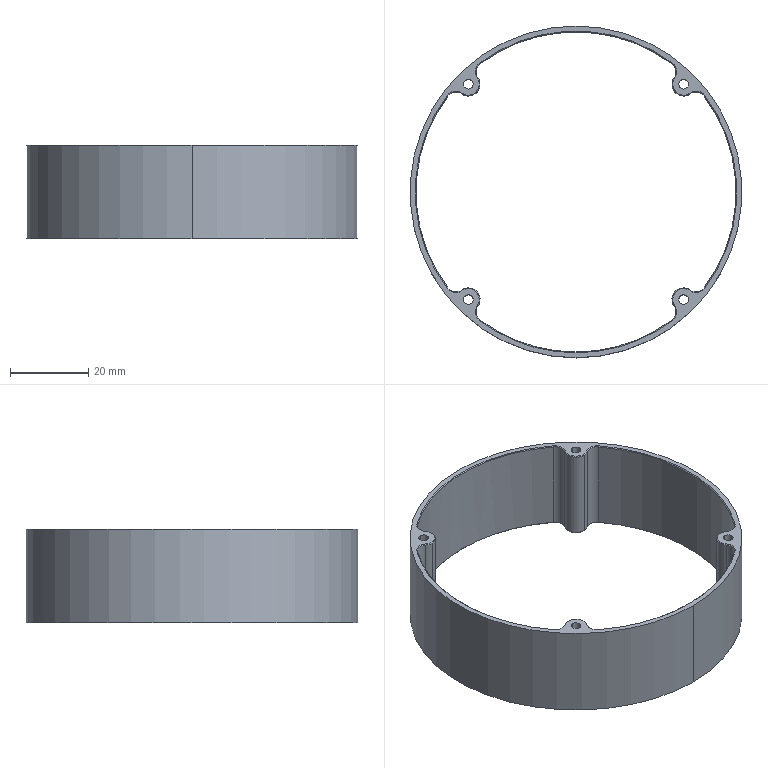NC program | NX | posted with a generic post | part box 85 x 85 x 24 mm
Whole program:
N10 G17 G21 G94 G90
(FLOOR_WALL , TOOL : D80)
N12 T19 M6
N14 G54
N16 G17 G0 G90 X-90.5 Y47.497 S6500 M3
N18 G43 Z30. H19
N20 Z3.
N22 G94 G1 Z0. F1500.
N24 X-87.5
N26 X87.5
N28 Y-15.5
N30 X-87.5
N32 X-90.5
N34 Z3.
N36 G0 Z30.
N38 M5
(ADAPTIVE_MILLING , TOOL : D10)
N40 T15 M6
N42 G54
N44 G17 G0 G90 X-55.209 Y0.813 S9500 M3
N46 G43 Z30. H15
N48 Z-21.
N50 G94 G1 Z-24. F1000.
N52 X-54.429 Y0.533 F3000.
N54 X-53.64 Y0.277
N56 G3 X-52.562 Y0.813 R1.017
N58 X-51.801 Y3.876 R8.28
N60 X-51.519 Y13.744 R111.643
N62 G1 X-51.514 Y15.994
N64 X-51.511 Y19.869
N66 X-51.51 Y33.494
N68 Y44.369
N70 X-51.509 Y44.494
N72 X-51.508 Y44.618
N74 G2 X-49.014 Y48.899 R5.714
N76 X-43.574 Y50.965 R12.318
N78 X-35.346 Y51.454 R58.245
N80 G1 X-34.346 Y51.464
N82 X-33.096 Y51.472
N84 X-31.347 Y51.48
N86 X-29.097 Y51.485
N88 X-25.222 Y51.487
N90 X-10.472 Y51.488
N92 X34.403
N94 X35.153 Y51.492
N96 X36.278 Y51.494
N98 X37.153
N100 X37.903 Y51.496
N102 X39.028
N104 G2 X45.027 Y51.463 R213.622
N106 X49.208 Y48.563 R6.076
N108 X51.082 Y42.786 R13.838
N110 X51.47 Y33.674 R81.696
N112 G1 X51.477 Y32.174
N114 X51.483 Y30.174
N116 X51.486 Y27.174
N118 X51.488 Y20.424
N120 Y-44.576
N122 X51.484 Y-44.701
N124 G2 X48.93 Y-48.952 R5.793
N126 X43.474 Y-50.979 R12.522
N128 X35.245 Y-51.455 R59.636
N130 G1 X34.12 Y-51.466
N132 X32.995 Y-51.473
N134 X31.495 Y-51.479
N136 X29.245 Y-51.484
N138 X25.495 Y-51.487
N140 X12.745 Y-51.488
N142 X-44.505
N144 X-44.63 Y-51.486
N146 X-44.755 Y-51.48
N148 X-44.879 Y-51.471
N150 G2 X-49.054 Y-48.781 R5.933
N152 X-51.022 Y-43.17 R12.937
N154 X-51.464 Y-34.313 R70.547
N156 G1 X-51.473 Y-33.063
N158 X-51.479 Y-31.438
N160 X-51.484 Y-29.063
N162 X-51.487 Y-25.188
N164 X-51.488 Y-11.938
N166 Y-2.938
N168 G2 X-50.952 Y2.659 R65.706
N170 G3 X-50.542 Y13.772 R121.144
N172 G1 X-50.534 Y15.397
N174 X-50.528 Y17.522
N176 X-50.523 Y20.647
N178 X-50.521 Y26.647
N180 Y41.397
N182 X-50.519 Y41.522
N184 G2 X-46.822 Y47.831 R7.658
N186 X-40.599 Y49.949 R15.406
N188 X-31.994 Y50.437 R67.483
N190 G1 X-30.869 Y50.449
N192 X-29.619 Y50.458
N194 X-27.994 Y50.466
N196 X-25.869 Y50.472
N198 X-22.619 Y50.476
N200 X-15.619 Y50.478
N202 X31.381
N204 X32.256 Y50.482
N206 X33.381 Y50.485
N208 X34.256
N210 X35.006 Y50.489
N212 X36.131 Y50.491
N214 G2 X42.254 Y50.449 R121.112
N216 X47.892 Y46.712 R7.759
N218 X49.996 Y40.224 R15.82
N220 X50.448 Y30.991 R77.748
N222 G1 X50.458 Y29.741
N224 X50.466 Y28.116
N226 X50.472 Y25.991
N228 X50.475 Y22.866
N230 X50.477 Y16.366
N232 X50.478 Y-41.384
N234 G2 X46.906 Y-47.756 R7.572
N236 X40.829 Y-49.911 R14.905
N238 X32.226 Y-50.433 R63.965
N240 G1 X31.226 Y-50.445
N242 X29.976 Y-50.455
N244 X28.476 Y-50.464
N246 X26.851 Y-50.469
N248 X24.227 Y-50.474
N250 X19.602 Y-50.477
N252 X-5.523 Y-50.478
N254 X-41.398
N256 X-41.523 Y-50.477
N258 X-41.648 Y-50.474
N260 X-41.773 Y-50.469
N262 X-41.898 Y-50.463
N264 G2 X-47.966 Y-46.571 R7.736
N266 X-49.986 Y-40.312 R16.029
N268 X-50.447 Y-30.954 R79.258
N270 G1 X-50.456 Y-29.829
N272 X-50.464 Y-28.454
N274 X-50.47 Y-26.454
N276 X-50.474 Y-23.704
N278 X-50.477 Y-18.704
N280 X-50.478 Y-5.329
N282 G2 X-49.974 Y2.402 R101.984
N284 G3 X-49.542 Y18.267 R208.612
N286 G1 X-49.536 Y21.017
N288 X-49.533 Y25.267
N290 X-49.532 Y36.142
N292 Y38.392
N294 X-49.53 Y38.767
N296 X-49.528 Y38.892
N298 G2 X-44.723 Y46.953 R8.987
N300 X-37.94 Y48.979 R18.304
N302 X-27.206 Y49.443 R96.865
N304 G1 X-25.706 Y49.451
N306 X-23.706 Y49.458
N308 X-20.956 Y49.463
N310 X-16.456 Y49.466
N312 X1.169 Y49.467
N314 X28.419
N316 G2 X39.793 Y49.452 R397.8
N318 X46.908 Y44.779 R8.926
N320 X48.996 Y37.758 R18.255
N322 X49.439 Y27.648 R96.534
N324 G1 X49.448 Y26.398
N326 X49.455 Y24.773
N328 X49.461 Y22.523
N330 X49.465 Y19.148
N332 X49.467 Y12.148
N334 Y-38.727
N336 G2 X44.822 Y-46.874 R8.92
N338 X37.934 Y-48.972 R17.859
N340 X27.451 Y-49.44 R95.726
N342 G1 X26.076 Y-49.449
N344 X24.326 Y-49.456
N346 X21.951 Y-49.462
N348 X18.201 Y-49.465
N350 X9.451 Y-49.467
N352 X-38.799
N354 G2 X-46.91 Y-44.755 R8.939
N356 X-48.964 Y-37.982 R17.998
N358 X-49.437 Y-27.749 R91.373
N360 G1 X-49.446 Y-26.624
N362 X-49.454 Y-24.999
N364 X-49.46 Y-22.874
N366 X-49.464 Y-19.874
N368 X-49.466 Y-14.124
N370 X-49.467 Y-7.124
N372 G2 X-49.015 Y1.737 R130.332
N374 G3 X-48.553 Y20.103 R271.383
N376 G1 X-48.547 Y23.103
N378 X-48.544 Y27.853
N380 X-48.542 Y35.353
N382 X-48.538 Y36.103
N384 X-48.531 Y36.728
N386 X-48.525 Y36.978
N388 G2 X-42.997 Y45.963 R9.907
N390 X-35.568 Y48.004 R20.654
N392 X-24.706 Y48.431 R112.646
N394 G1 X-23.081 Y48.44
N396 X-21.081 Y48.447
N398 X-18.331 Y48.452
N400 X-13.956 Y48.455
N402 X-0.706 Y48.456
N404 X25.419
N406 G2 X37.793 Y48.44 R387.041
N408 X45.938 Y43.012 R9.811
N410 X47.951 Y35.961 R20.187
N412 X48.43 Y24.727 R104.006
N414 G1 X48.44 Y23.102
N416 X48.446 Y21.477
N418 X48.451 Y19.102
N420 X48.455 Y15.102
N422 X48.456 Y5.227
N424 Y-36.398
N426 G2 X46.892 Y-42.473 R10.44
N428 X40.838 Y-46.879 R11.611
N430 X32.851 Y-48.224 R29.907
N432 X17.98 Y-48.452 R295.19
N434 G1 X13.105 Y-48.455
N436 X-6.645 Y-48.456
N438 X-36.395
N440 X-36.645 Y-48.455
N442 X-37.02 Y-48.449
N444 X-37.145 Y-48.446
N446 G2 X-45.927 Y-43.01 R9.838
N448 X-47.963 Y-35.837 R20.191
N450 X-48.43 Y-24.728 R104.118
N452 X-48.396 Y-5.229 R799.482
N454 G3 X-47.66 Y10.378 R561.193
N456 X-47.554 Y32.377 R970.189
N458 G2 X-47.312 Y37.365 R30.793
N460 X-41.626 Y44.852 R10.503
N462 X-33.958 Y46.962 R21.44
N464 X-22.597 Y47.418 R115.711
N466 G1 X-20.847 Y47.428
N468 X-18.847 Y47.436
N470 X-16.097 Y47.441
N472 X-11.722 Y47.444
N474 X-4.297 Y47.445
N476 X-4.061 Y47.476
N478 X-4.016 Y47.48
N480 X0.03 Y47.65
N482 G3 X9.915 Y47.471 R166.471
N484 G1 X13.665 Y47.468
N486 X26.165 Y47.467
N488 X29.165
N490 X30.04 Y47.472
N492 X31.165 Y47.474
N494 X31.79 Y47.475
N496 G2 X37.156 Y47.296 R36.852
N498 X44.872 Y41.551 R10.436
N500 X46.934 Y34.125 R21.464
N502 X47.417 Y22.891 R107.945
N504 G1 X47.426 Y21.391
N506 X47.434 Y19.516
N508 X47.44 Y17.016
N510 X47.443 Y13.141
N512 X47.445 Y4.891
N514 Y3.879
N516 X47.625 Y1.516
N518 X47.626 Y1.481
N520 G3 X47.468 Y-15.514 R828.65
N522 G1 X47.467 Y-27.764
N524 Y-33.389
N526 X47.463 Y-34.139
N528 X47.457 Y-34.639
N530 X47.451 Y-35.014
N532 X47.443 Y-35.264
N534 G2 X41.334 Y-44.978 R10.59
N536 X33.76 Y-46.978 R22.282
N538 X21.649 Y-47.424 R126.599
N540 G1 X19.899 Y-47.432
N542 X17.524 Y-47.438
N544 X14.024 Y-47.443
N546 X7.399 Y-47.445
N548 X4.365
N550 X4.288 Y-47.456
N552 X4.241 Y-47.46
N554 X0.031 Y-47.65
N556 G3 X-10.227 Y-47.469 R173.888
N558 G1 X-16.227 Y-47.467
N560 X-33.352
N562 X-34.102 Y-47.463
N564 X-34.727 Y-47.456
N566 X-34.852 Y-47.454
N568 X-35.102 Y-47.448
N570 G2 X-42.248 Y-44.919 R10.74
N572 X-46.125 Y-38.333 R13.491
N574 X-47.278 Y-29.553 R38.681
N576 X-47.35 Y-4.931 R510.076
N578 G1 X-47.531 Y-3.357
N580 X-47.534 Y-3.31
N582 X-47.642 Y0.863
N584 X-47.641 Y0.889
N586 X-47.381 Y5.048
N588 X-47.376 Y5.095
N590 G3 X-46.645 Y13.929 R52.853
N592 G1 X-46.629 Y14.804
N594 X-46.615 Y15.804
N596 X-46.602 Y17.053
N598 X-46.591 Y18.553
N600 X-46.582 Y20.303
N602 X-46.575 Y22.428
N604 X-46.569 Y25.428
N606 X-46.565 Y29.553
N608 X-46.55 Y31.678
N610 X-46.542 Y32.553
N612 X-46.539 Y32.803
N614 X-46.53 Y33.178
N616 X-46.518 Y33.553
N618 G2 X-44.226 Y40.555 R11.578
N620 X-37.754 Y44.833 R13.23
N622 X-29.511 Y46.179 R33.266
N624 X-15.64 Y46.427 R273.643
N626 G1 X-12.265 Y46.432
N628 X-10.64 Y46.433
N630 X-10.515 Y46.437
N632 X-10.488 Y46.439
N634 X-8.1 Y46.955
N636 X-8.056 Y46.963
N638 X-4.212 Y47.456
N640 X-4.016 Y47.48
N642 X0.043 Y47.649
N644 X4.344 Y47.45
N646 X4.392 Y47.446
N648 G3 X11.384 Y46.618 R79.329
N650 X27.007 Y46.478 R436.443
N652 G2 X34.63 Y46.393 R128.069
N654 X43.811 Y40.169 R11.019
N656 X45.915 Y32.495 R22.346
N658 X46.408 Y20.511 R118.097
N660 G1 X46.417 Y18.886
N662 X46.424 Y16.886
N664 X46.43 Y14.136
N666 X46.433 Y10.761
N668 X46.435 Y10.636
N670 X46.447 Y10.528
N672 X46.604 Y9.926
N674 X46.614 Y9.879
N676 X47.301 Y5.745
N678 X47.307 Y5.698
N680 X47.449 Y3.829
N682 G3 X48.993 Y3.067 R1.002
N684 X49.45 Y3.73 Z-23.959 R1.196
N686 G1 X49.872 Y4.829 Z-23.9
N688 X50.603 Y6.759
N690 X50.631 Y7.011
N692 X50.584 Y10.383
N694 X50.49 Y13.754
N696 X50.365 Y15.999
N698 X50.198 Y18.24
N700 X48.844 Y33.808
N702 G3 X45.583 Y43.122 R20.156
N704 G1 X44.85 Y44.128
N706 X43.43 Y45.921
N708 G3 X40.99 Y47.729 R7.825
N710 G1 X40.309 Y48.033
N712 X39.61 Y48.295
N714 X38.272 Y48.736
N716 X36.918 Y49.127
N718 G3 X32.914 Y49.653 R18.329
N720 G1 X11.828 Y50.04
N722 X11.629 Y50.02
N724 X11.436 Y49.968
N726 X9.587 Y49.224
N728 X8.947 Y48.971 Z-23.934
N730 X8.315 Y48.7 Z-23.969
N732 G3 X7.91 Y48.239 Z-24. R1.045
N734 X8.646 Y46.858 R1.003
N736 X13.46 Y45.84 R49.887
N738 X23.199 Y45.502 R97.139
N740 G2 X32.822 Y45.403 R225.532
N742 X42.81 Y38.743 R11.531
N744 X44.88 Y31.058 R23.133
N746 X45.385 Y19.949 R108.532
N748 G3 X45.448 Y14.279 R127.609
N750 G1 X45.537 Y14.028
N752 X45.551 Y13.982
N754 X46.462 Y10.474
N756 G3 X48.353 Y10.341 R1.001
N758 G1 X48.425 Y10.639 Z-23.985
N760 X48.449 Y10.944 Z-23.969
N762 X48.556 Y12.326 Z-23.9
N764 X48.712 Y14.371
N766 X48.717 Y19.057
N768 X48.697 Y23.743
N770 G3 X47.992 Y31.186 R53.686
N772 G1 X47.702 Y32.931
N774 X47.365 Y34.667
N776 G3 X46.205 Y38.528 R28.82
N778 X43.793 Y42.748 R17.948
N780 X40.724 Y45.809 R14.618
N782 X36.241 Y47.859 R10.519
N784 X31.923 Y48.423 R28.426
N786 G1 X15.284 Y49.238
N788 X15.064 Y49.221
N790 X14.851 Y49.163
N792 X13.062 Y48.418
N794 X12.429 Y48.159 Z-23.934
N796 X11.804 Y47.882 Z-23.968
N798 G3 X11.403 Y47.407 Z-24. R1.044
N800 X12.102 Y46.056 R1.004
N802 G2 X14.944 Y45.213 R33.167
N804 G3 X21.528 Y44.584 R33.194
N806 G2 X31.275 Y44.406 R382.287
N808 X39.687 Y40.563 R11.931
N810 X43.243 Y33.217 R16.321
N812 X44.258 Y23.912 R49.518
N814 G1 X44.279 Y23.287
N816 X44.3 Y22.538
N818 X44.318 Y21.788
N820 X44.338 Y20.788
N822 X44.355 Y19.788
N824 X44.368 Y18.788
N826 X44.381 Y17.413
N828 X44.393 Y17.289
N830 X44.417 Y17.166
N832 X45.468 Y14.223
N834 G3 X47.184 Y13.926 R1.002
N836 X47.422 Y14.659 Z-23.961 R1.192
N838 G1 X47.527 Y15.869 Z-23.9
N840 X47.718 Y18.12
N842 X47.705 Y22.939
N844 G3 X47.101 Y29.319 R46.054
N846 G1 X46.452 Y33.137
N848 G3 X43.336 Y40.694 R21.206
N850 X41.392 Y43.341 R31.022
N852 X39.825 Y44.651 R6.807
N854 X36.587 Y46.328 R31.493
N856 X33.516 Y47.108 R10.675
N858 X17.765 Y48.495 R577.882
N860 G1 X17.519 Y48.481
N862 X17.282 Y48.413
N864 X15.548 Y47.645
N866 X14.941 Y47.381 Z-23.933
N868 X14.344 Y47.096 Z-23.966
N870 G3 X13.945 Y46.566 Z-24. R1.039
N872 X14.583 Y45.313 R1.005
N874 X18.614 Y44.088 R33.85
N876 X25.463 Y43.578 R46.475
N878 G2 X31.572 Y43.216 R45.964
N880 X40.667 Y36.327 R12.184
N882 X42.832 Y28.28 R24.357
N884 X43.33 Y19.798 R99.797
N886 G3 X44.129 Y17.975 R18.027
N888 G1 X44.423 Y17.151
N890 G3 X46.137 Y16.851 R1.002
N892 X46.378 Y17.599 Z-23.96 R1.214
N894 G1 X46.481 Y18.793 Z-23.9
N896 X46.673 Y21.048
N898 X46.659 Y23.67
N900 G3 X46.337 Y26.642 R21.691
N902 G1 X45.874 Y29.204
N904 X45.393 Y31.762
N906 G3 X43.469 Y37.456 R27.489
N908 X41.841 Y40.097 R17.347
N910 X39.938 Y42.405 R20.339
N912 X37.858 Y43.975 R10.921
N914 X33.985 Y45.758 R16.965
N916 X29.291 Y46.78 R21.13
N918 G1 X20.225 Y47.679
N920 G3 X19.699 Y47.587 R1.061
N922 G1 X18.046 Y46.806
N924 X17.451 Y46.53 Z-23.933
N926 X16.867 Y46.231 Z-23.966
N928 G3 X16.479 Y45.68 Z-24. R1.039
N930 X17.043 Y44.497 R1.005
N932 X20.553 Y43.203 R16.713
N934 X26.518 Y42.614 R41.775
N936 G2 X32.426 Y41.694 R21.487
N938 X39.73 Y34.908 R12.64
N940 X41.851 Y26.59 R25.864
N942 G1 X42.194 Y22.229
N944 G3 X43.403 Y19.554 R39.058
N946 X44.95 Y19.202 R1.003
N948 X45.326 Y20.054 Z-23.952 R1.138
N950 G1 X45.437 Y21.087 Z-23.9
N952 X45.666 Y23.316
N954 X45.653 Y23.451
N956 X45.163 Y26.41
N958 X44.653 Y29.365
N960 G3 X43.164 Y34.565 R30.507
N962 X41.552 Y37.719 R20.614
N964 G1 X40.214 Y39.824
N966 G3 X39.226 Y41.023 R7.006
N968 X37.021 Y42.755 R30.123
N970 X32.525 Y44.812 R14.108
N972 G1 X31.614 Y45.002
N974 X30.694 Y45.145
N976 G3 X25.736 Y45.711 R78.112
N978 G1 X22.685 Y45.951
N980 X20.484 Y45.738
N982 X19.745 Y45.672 Z-23.937
N984 X19.009 Y45.578 Z-23.974
N986 X18.774 Y45.475 Z-23.987
N988 X18.569 Y45.321 Z-24.
N990 G3 X18.877 Y43.698 R1.002
N992 X22.284 Y42.353 R22.767
N994 X27.722 Y41.552 R54.397
N996 G2 X34.936 Y38.661 R14.117
N998 X39.571 Y31.527 R15.097
N1000 X40.935 Y24.421 R34.74
N1002 G1 X40.966 Y24.299
N1004 X41.008 Y24.182
N1006 X41.017 Y24.159
N1008 X42.325 Y21.884
N1010 G3 X43.737 Y21.544 R1.004
N1012 X44.196 Y22.341 Z-23.952 R1.045
N1014 G1 X44.337 Y23.378 Z-23.9
N1016 X44.487 Y24.438
N1018 X44.617 Y25.501
N1020 X44.575 Y25.781
N1022 X43.771 Y28.473
N1024 X42.929 Y31.153
N1026 G3 X41.373 Y35.098 R30.719
N1028 G1 X40.792 Y36.221
N1030 X40.193 Y37.336
N1032 G3 X37.302 Y40.664 R12.597
N1034 X35.274 Y42.103 R17.249
N1036 G1 X34.212 Y42.742
N1038 X33.123 Y43.334
N1040 G3 X28.416 Y44.673 R14.078
N1042 G1 X24.773 Y45.037
N1044 X22.527 Y44.803
N1046 X21.843 Y44.734 Z-23.934
N1048 X21.161 Y44.645 Z-23.969
N1050 G3 X20.645 Y44.311 Z-24. R1.045
N1052 X20.979 Y42.782 R1.003
N1054 X25.798 Y40.994 R13.052
N1056 G2 X31.616 Y39.154 R21.183
N1058 X37.982 Y31.87 R14.116
N1060 X39.457 Y26.711 R28.047
N1062 G3 X40.195 Y25.589 R10.243
N1064 G1 X41.067 Y24.072
N1066 G3 X42.921 Y24.412 R1.001
N1068 G1 X42.92 Y24.729 Z-23.984
N1070 X42.863 Y25.041 Z-23.968
N1072 X42.613 Y26.382 Z-23.9
N1074 X42.232 Y28.419
N1076 X41.582 Y30.96
N1078 G3 X40.536 Y33.759 R20.782
N1080 G1 X39.284 Y36.443
N1082 G3 X37.294 Y38.969 R8.965
N1084 X33.726 Y41.466 R20.868
N1086 X29.167 Y43.428 R20.809
N1088 G1 X27.636 Y43.884
N1090 X26.099 Y44.318
N1092 X25.822 Y44.321
N1094 X23.877 Y44.064
N1096 X23.203 Y43.979 Z-23.934
N1098 X22.532 Y43.873 Z-23.968
N1100 G3 X22.016 Y43.512 Z-24. R1.043
N1102 X22.338 Y42.039 R1.004
N1104 X27.686 Y39.642 R25.44
N1106 G2 X37.228 Y30.071 R15.257
N1108 G3 X37.698 Y29.142 R2.391
N1110 G1 X39.568 Y26.484
N1112 G3 X41.258 Y26.57 R1.002
N1114 X41.345 Y27.4 Z-23.957 R1.173
N1116 G1 X41.171 Y28.532 Z-23.9
N1118 X40.845 Y30.582
N1120 X40.733 Y30.83
N1122 X38.962 Y33.651
N1124 X37.17 Y36.457
N1126 G3 X34.435 Y39.25 R12.493
N1128 X31.971 Y40.937 R27.195
N1130 G1 X28.207 Y43.206
N1132 G3 X27.515 Y43.334 R1.031
N1134 G1 X25.778 Y43.024
N1136 X25.116 Y42.911 Z-23.934
N1138 X24.458 Y42.775 Z-23.967
N1140 G3 X23.952 Y42.377 Z-24. R1.041
N1142 X24.31 Y40.956 R1.004
N1144 G2 X26.914 Y39.292 R54.476
N1146 X32.014 Y35.71 R24.969
N1148 X34.102 Y33.227 R17.672
N1150 G1 X34.856 Y32.488
N1152 X34.889 Y32.453
N1154 X37.56 Y29.309
N1156 G3 X39.144 Y30.83 R-1.1
N1158 G1 X27.743 Y41.342
N1160 G3 X26.383 Y39.621 R-1.1
N1162 G1 X28.388 Y38.269
N1164 X28.427 Y38.24
N1166 X31.754 Y35.526
N1168 X31.79 Y35.494
N1170 X34.111 Y33.219
N1172 G3 X35.042 Y32.96 R1.014
N1174 G1 X35.333 Y33.029
N1176 X37.279 Y33.491 Z-23.9
N1178 X37.595 Y33.566
N1180 X37.919 Y33.59
N1182 G2 X38.611 Y33.219 R1.026
N1184 G1 X39.665 Y31.903
N1186 X40.681 Y30.558
N1188 X41.304 Y29.624
N1190 X41.891 Y28.667
N1192 X44.567 Y24.01
N1194 G2 X48.806 Y13.376 R45.825
N1196 X50.336 Y5.112 R56.19
N1198 X50.751 Y0.417 R90.539
N1200 X50.312 Y-0.485 R1.011
N1202 G1 X50.115 Y-0.617
N1204 X48.456 Y-1.734 Z-24.
N1206 X47.89 Y-2.128
N1208 G3 X47.569 Y-2.765 R1.031
N1210 G1 X47.142 Y-6.935
N1212 X47.135 Y-6.981
N1214 G3 X46.542 Y-13.443 R32.952
N1216 X46.471 Y-31.568 R950.255
N1218 G2 X45.986 Y-36.904 R20.474
N1220 X39.989 Y-43.895 R11.107
N1222 X32.545 Y-45.906 R22.561
N1224 X20.811 Y-46.404 R113.834
N1226 G1 X19.311 Y-46.414
N1228 X17.561 Y-46.421
N1230 X15.186 Y-46.428
N1232 X11.811 Y-46.432
N1234 X10.561 Y-46.433
N1236 X10.448 Y-46.442
N1238 X8.488 Y-46.887
N1240 X8.442 Y-46.895
N1242 X4.354 Y-47.447
N1244 G3 X3.592 Y-48.883 R1.003
N1246 X4.303 Y-49.44 Z-23.954 R1.156
N1248 G1 X5.299 Y-49.831 Z-23.9
N1250 X7.278 Y-50.599
N1252 X7.536 Y-50.629
N1254 X10.658 Y-50.577
N1256 X13.779 Y-50.473
N1258 X15.337 Y-50.378
N1260 X16.894 Y-50.266
N1262 X33.09 Y-48.916
N1264 G3 X41.436 Y-46.55 R22.96
N1266 X43.559 Y-45.25 R18.557
N1268 G1 X45.415 Y-43.913
N1270 G3 X47.649 Y-41.174 R8.864
N1272 X48.828 Y-37.903 R12.733
N1274 X49.408 Y-33.59 R22.476
N1276 G1 X50.103 Y-11.268
N1278 X50.084 Y-11.061
N1280 X50.03 Y-10.861
N1282 X49.299 Y-9.057
N1284 X49.039 Y-8.408 Z-23.935
N1286 X48.763 Y-7.765 Z-23.97
N1288 G3 X48.323 Y-7.368 Z-24. R1.048
N1290 X46.921 Y-8.086 R1.003
N1292 G2 X45.977 Y-12.599 R89.393
N1294 G3 X45.528 Y-20.079 R52.172
N1296 G2 X45.424 Y-32.327 R757.959
N1298 X42.763 Y-39.71 R11.879
N1300 X36.058 Y-43.871 R14.05
N1302 X27.179 Y-45.196 R36.723
N1304 X14.307 Y-45.422 R319.17
N1306 X10.381 Y-46.457 R32.304
N1308 G3 X10.359 Y-48.403 R1.001
N1310 G1 X11.115 Y-48.48 Z-23.962
N1312 X11.872 Y-48.53 Z-23.924
N1314 X12.352 Y-48.566 Z-23.9
N1316 X14.278 Y-48.707
N1318 X18.652 Y-48.712
N1320 X23.025 Y-48.695
N1322 G3 X31.71 Y-47.885 R61.155
N1324 G1 X33.56 Y-47.579
N1326 X35.407 Y-47.256
N1328 G3 X39.703 Y-45.671 R16.45
N1330 G1 X40.676 Y-45.119
N1332 X41.621 Y-44.52
N1334 X42.577 Y-43.874
N1336 X43.503 Y-43.186
N1338 G3 X45.734 Y-40.792 R13.301
N1340 X47.494 Y-37.514 R12.035
N1342 X48.279 Y-33.874 R12.656
N1344 G1 X49.337 Y-14.925
N1346 X49.32 Y-14.696
N1348 X49.258 Y-14.475
N1350 X48.498 Y-12.703
N1352 X48.239 Y-12.086 Z-23.933
N1354 X47.958 Y-11.479 Z-23.967
N1356 G3 X47.449 Y-11.076 Z-24. R1.041
N1358 X46.155 Y-11.743 R1.004
N1360 X44.975 Y-16.211 R41.294
N1362 X44.54 Y-23.943 R58.969
N1364 G2 X44.366 Y-31.689 R125.388
N1366 X37.52 Y-41.726 R11.892
N1368 X29.594 Y-43.857 R23.88
N1370 X17.486 Y-44.38 R116.078
N1372 G3 X16.609 Y-44.66 R2.849
N1374 G1 X14.111 Y-45.466
N1376 G3 X13.85 Y-47.241 R1.002
N1378 X14.532 Y-47.431 Z-23.964 R1.267
N1380 G1 X15.809 Y-47.537 Z-23.9
N1382 X18.008 Y-47.716
N1384 X22.827 Y-47.704
N1386 G3 X29.207 Y-47.1 R46.054
N1388 G1 X33.026 Y-46.451
N1390 G3 X41.26 Y-43.013 R23.251
N1392 X43.333 Y-41.417 R26.893
N1394 X45.836 Y-37.761 R9.416
N1396 X47.219 Y-32.672 R22.037
N1398 G1 X47.403 Y-31.283
N1400 X47.538 Y-29.888
N1402 X48.404 Y-18.168
N1404 X48.39 Y-17.929
N1406 X48.325 Y-17.698
N1408 X47.566 Y-15.94
N1410 X47.305 Y-15.325 Z-23.933
N1412 X47.023 Y-14.72 Z-23.967
N1414 G3 X46.511 Y-14.318 Z-24. R1.04
N1416 X45.222 Y-14.986 R1.004
N1418 X44.182 Y-18.048 R26.542
N1420 X43.584 Y-25.138 R40.613
N1422 G2 X43.222 Y-31.498 R49.008
N1424 X36.386 Y-40.629 R12.158
N1426 X28.47 Y-42.804 R24.075
N1428 X19.864 Y-43.323 R95.026
N1430 G3 X17.135 Y-44.44 R27.003
N1432 X16.801 Y-46.049 R1.002
N1434 X17.629 Y-46.374 Z-23.954 R1.165
N1436 G1 X18.709 Y-46.476 Z-23.9
N1438 X21.032 Y-46.69
N1440 X23.655 Y-46.676
N1442 G3 X26.627 Y-46.354 R21.691
N1444 G1 X29.188 Y-45.891
N1446 X31.746 Y-45.41
N1448 G3 X37.441 Y-43.486 R27.489
N1450 X40.082 Y-41.858 R17.347
N1452 X42.389 Y-39.955 R20.347
N1454 X43.96 Y-37.875 R10.938
N1456 X45.747 Y-34.003 R17.001
N1458 X46.774 Y-29.308 R21.169
N1460 G1 X47.705 Y-20.029
N1462 G3 X47.619 Y-19.51 R1.064
N1464 G1 X46.845 Y-17.832
N1466 X46.574 Y-17.231 Z-23.933
N1468 X46.28 Y-16.641 Z-23.966
N1470 G3 X45.74 Y-16.248 Z-24. R1.039
N1472 X44.523 Y-16.847 R1.005
N1474 X43.22 Y-20.561 R26.6
N1476 X42.612 Y-26.523 R39.431
N1478 G2 X41.687 Y-32.431 R21.598
N1480 X35.12 Y-39.62 R12.586
N1482 X26.824 Y-41.819 R25.339
N1484 X22.091 Y-42.207 R260.62
N1486 G3 X20.512 Y-43.008 R18.379
N1488 G1 X19.591 Y-43.398
N1490 G3 X19.241 Y-44.991 R1.003
N1492 X20.074 Y-45.334 Z-23.954 R1.157
N1494 G1 X21.142 Y-45.443 Z-23.9
N1496 X23.356 Y-45.661
N1498 X26.382 Y-45.173
N1500 X29.403 Y-44.648
N1502 G3 X34.602 Y-43.159 R30.507
N1504 X37.756 Y-41.547 R20.614
N1506 G1 X39.862 Y-40.209
N1508 G3 X41.06 Y-39.22 R6.965
N1510 X42.788 Y-37.012 R29.823
N1512 X44.863 Y-32.336 R13.812
N1514 G1 X45.053 Y-31.29
N1516 X45.351 Y-29.127
N1518 X45.611 Y-26.96
N1520 X45.77 Y-24.992
N1522 X45.893 Y-23.02
N1524 X45.89 Y-22.861
N1526 X45.677 Y-20.686
N1528 X45.611 Y-19.983 Z-23.935
N1530 X45.529 Y-19.283 Z-23.971
N1532 G3 X45.231 Y-18.785 Z-24. R1.05
N1534 X43.643 Y-19.123 R1.003
N1536 X41.909 Y-24.738 R13.732
N1538 G2 X40.995 Y-30.407 R36.091
N1540 X33.844 Y-38.634 R12.99
N1542 X25.288 Y-40.829 R26.292
N1544 G3 X24.253 Y-41.015 R3.997
N1546 G1 X21.826 Y-42.309
N1548 G3 X21.473 Y-43.758 R1.004
N1550 X22.263 Y-44.196 Z-23.953 R1.047
N1552 G1 X23.319 Y-44.333 Z-23.9
N1554 X24.382 Y-44.476
N1556 X25.447 Y-44.601
N1558 X25.723 Y-44.559
N1560 G3 X33.459 Y-42.098 R149.068
N1562 X37.329 Y-40.305 R21.978
N1564 X40.231 Y-37.851 R13.356
N1566 X43.411 Y-33.361 R19.421
N1568 X44.624 Y-29.171 R12.472
N1570 G1 X45.106 Y-24.528
N1572 X44.875 Y-22.316
N1574 X44.803 Y-21.619 Z-23.935
N1576 X44.715 Y-20.925 Z-23.97
N1578 G3 X44.403 Y-20.424 Z-24. R1.048
N1580 X42.85 Y-20.736 R1.003
N1582 X41.443 Y-23.934 R18.984
N1584 G2 X40.28 Y-28.795 R350.224
N1586 X32.137 Y-37.866 R13.825
N1588 X26.631 Y-39.483 R29.99
N1590 G1 X26.522 Y-39.534
N1592 X24.293 Y-40.991
N1594 X24.253 Y-41.015
N1596 G3 X24.437 Y-42.821 R1.001
N1598 X25.139 Y-42.823 Z-23.964 R1.275
N1600 G1 X26.405 Y-42.588 Z-23.9
N1602 X28.599 Y-42.18
N1604 X31.14 Y-41.53
N1606 G3 X35.604 Y-39.654 R22.45
N1608 X38.523 Y-37.385 R13.741
N1610 G1 X39.57 Y-36.314
N1612 X40.605 Y-35.23
N1614 G3 X42.366 Y-32.246 R10.262
N1616 G1 X42.696 Y-31.306
N1618 X44.161 Y-26.539
N1620 X44.197 Y-26.332
N1622 Y-26.121
N1624 X43.953 Y-24.175
N1626 X43.871 Y-23.491 Z-23.935
N1628 X43.769 Y-22.808 Z-23.969
N1630 G3 X43.43 Y-22.301 Z-24. R1.045
N1632 X41.911 Y-22.642 R1.003
N1634 X40.711 Y-24.819 R40.578
N1636 G2 X38.939 Y-29.358 R112.032
N1638 X30.357 Y-37.115 R15.057
N1640 G1 X30.123 Y-37.204
N1642 X29.888 Y-37.29
N1644 X29.535 Y-37.416
N1646 X29.419 Y-37.462
N1648 X29.308 Y-37.519
N1650 X29.272 Y-37.54
N1652 G2 X26.441 Y-39.587 R24.111
N1654 G3 X26.573 Y-41.334 R1.002
N1656 X27.331 Y-41.382 Z-23.961 R1.201
N1658 G1 X28.542 Y-41.19 Z-23.9
N1660 X30.543 Y-40.863
N1662 X30.788 Y-40.752
N1664 X33.608 Y-38.981
N1666 X36.415 Y-37.189
N1668 G3 X39.211 Y-34.457 R12.556
N1670 X40.9 Y-31.994 R26.778
N1672 G1 X43.348 Y-27.932
N1674 G3 X43.475 Y-27.23 R1.031
N1676 G1 X43.149 Y-25.505
N1678 X43.032 Y-24.854 Z-23.933
N1680 X42.89 Y-24.207 Z-23.966
N1682 G3 X42.467 Y-23.697 Z-24. R1.039
N1684 X41.098 Y-24.035 R1.005
N1686 G2 X37.264 Y-30.172 R121.565
N1688 X33.217 Y-34.106 R16.611
N1690 X29.265 Y-37.545 R35.447
N1692 G3 X30.749 Y-39.162 R-1.1
N1694 G1 X41.23 Y-27.992
N1696 G3 X39.543 Y-26.586 R-1.1
N1698 G1 X37.053 Y-29.958
N1700 X37.024 Y-29.994
N1702 X34.245 Y-33.132
N1704 X34.212 Y-33.166
N1706 X33.213 Y-34.11
N1708 G3 X32.929 Y-35.08 R1.011
N1710 G1 X32.996 Y-35.347
N1712 X33.483 Y-37.286 Z-23.9
N1714 X33.559 Y-37.594
N1716 X33.585 Y-37.909
N1718 G2 X33.213 Y-38.61 R1.026
N1720 G1 X31.897 Y-39.664
N1722 X30.552 Y-40.68
N1724 X29.618 Y-41.303
N1726 X28.66 Y-41.89
N1728 X24.004 Y-44.566
N1730 G2 X12.907 Y-48.995 R48.663
N1732 X5.293 Y-50.358 R62.706
N1734 X1.822 Y-50.638 R38.943
N1736 G1 X0.079 Y-50.696
N1738 G2 X-0.867 Y-50.129 R1.061
N1740 G1 X-1.976 Y-48.465 Z-24.
N1742 X-2.411 Y-47.835
N1744 G3 X-3.103 Y-47.514 R1.027
N1746 G1 X-4.149 Y-47.468
N1748 X-4.195 Y-47.464
N1750 G3 X-10.976 Y-46.643 R105.277
N1752 X-24.348 Y-46.479 R298.94
N1754 G2 X-34.347 Y-46.397 R234.872
N1756 X-43.908 Y-39.955 R11.084
N1758 X-45.937 Y-32.26 R22.831
N1760 X-46.407 Y-20.525 R118.526
N1762 G1 X-46.416 Y-18.9
N1764 X-46.424 Y-16.775
N1766 X-46.429 Y-14.15
N1768 X-46.432 Y-10.65
N1770 X-46.438 Y-10.515
N1772 G2 X-47.356 Y-4.882 R38.736
N1774 G3 X-48.824 Y-4.116 R1.002
N1776 X-49.353 Y-4.819 Z-23.955 R1.172
N1778 G1 X-49.751 Y-5.84 Z-23.9
N1780 X-50.509 Y-7.809
N1782 X-50.538 Y-8.064
N1784 X-50.491 Y-11.436
N1786 X-50.397 Y-14.807
N1788 X-50.271 Y-17.051
N1790 X-50.105 Y-19.293
N1792 X-48.859 Y-33.616
N1794 G3 X-47.867 Y-38.49 R21.356
N1796 X-46.88 Y-40.772 R16.927
N1798 G1 X-46.176 Y-42.113
N1800 X-45.456 Y-43.446
N1802 G3 X-43.426 Y-45.874 R10.188
N1804 X-39.78 Y-48.222 R12.195
N1806 X-35.562 Y-49.247 R13.37
N1808 X-31.828 Y-49.502 R50.602
N1810 G1 X-11.548 Y-50.091
N1812 X-11.34 Y-50.071
N1814 X-11.138 Y-50.016
N1816 X-9.332 Y-49.273
N1818 X-8.694 Y-49.016 Z-23.934
N1820 X-8.064 Y-48.739 Z-23.969
N1822 G3 X-7.663 Y-48.274 Z-24. R1.045
N1824 X-8.366 Y-46.909 R1.003
N1826 X-13.504 Y-45.843 R61.329
N1828 X-22.493 Y-45.506 R88.154
N1830 G2 X-32.866 Y-45.387 R234.974
N1832 X-42.827 Y-38.686 R11.541
N1834 X-44.887 Y-30.996 R23.549
N1836 X-45.386 Y-19.763 R109.746
N1838 G1 X-45.397 Y-18.388
N1840 X-45.407 Y-16.638
N1842 X-45.414 Y-14.513
N1844 Y-14.388
N1846 X-45.427 Y-14.263
N1848 X-45.433 Y-14.225
N1850 G2 X-46.439 Y-10.509 R31.201
N1852 G3 X-48.397 Y-10.503 R1.
N1854 G1 X-48.552 Y-12.497 Z-23.9
N1856 X-48.689 Y-14.406
N1858 X-48.694 Y-19.092
N1860 X-48.674 Y-23.778
N1862 G3 X-47.97 Y-31.222 R53.686
N1864 G1 X-47.68 Y-32.966
N1866 X-47.342 Y-34.703
N1868 G3 X-46.182 Y-38.564 R28.82
N1870 X-43.77 Y-42.784 R17.948
N1872 X-40.7 Y-45.844 R14.587
N1874 X-36.215 Y-47.887 R10.485
N1876 X-31.895 Y-48.443 R28.479
N1878 G1 X-15.451 Y-49.217
N1880 X-15.233 Y-49.2
N1882 X-15.021 Y-49.142
N1884 X-13.215 Y-48.395
N1886 X-12.585 Y-48.138 Z-23.934
N1888 X-11.963 Y-47.863 Z-23.968
N1890 G3 X-11.559 Y-47.382 Z-24. R1.043
N1892 X-12.269 Y-46.035 R1.004
N1894 X-15.709 Y-45.049 R37.241
N1896 X-23.435 Y-44.547 R50.925
N1898 G2 X-31.681 Y-44.362 R141.71
N1900 X-41.832 Y-37.296 R11.951
N1902 X-43.916 Y-29.098 R25.031
N1904 X-44.381 Y-17.362 R124.554
N1906 G3 X-45.008 Y-15.642 R9.615
N1908 G1 X-45.438 Y-14.205
N1910 G3 X-47.255 Y-13.979 R1.001
N1912 X-47.409 Y-14.603 Z-23.968 R1.315
N1914 G1 X-47.518 Y-15.948 Z-23.9
N1916 X-47.688 Y-18.102
N1918 X-47.676 Y-22.921
N1920 G3 X-47.072 Y-29.301 R46.054
N1922 G1 X-46.423 Y-33.119
N1924 G3 X-43.307 Y-40.676 R21.206
N1926 X-41.312 Y-43.387 R31.452
N1928 X-37.68 Y-45.92 R9.225
N1930 X-32.579 Y-47.237 R19.379
N1932 G1 X-31.185 Y-47.402
N1934 X-29.788 Y-47.537
N1936 X-17.796 Y-48.487
N1938 X-17.551 Y-48.473
N1940 X-17.314 Y-48.405
N1942 X-15.577 Y-47.641
N1944 X-14.968 Y-47.378 Z-23.933
N1946 X-14.368 Y-47.093 Z-23.967
N1948 G3 X-13.968 Y-46.57 Z-24. R1.04
N1950 X-14.614 Y-45.305 R1.004
N1952 X-17.899 Y-44.234 R145.321
N1954 X-24.733 Y-43.595 R36.13
N1956 G2 X-31.22 Y-43.26 R59.936
N1958 X-40.617 Y-36.408 R12.179
N1960 X-42.823 Y-28.373 R24.122
N1962 X-43.329 Y-19.891 R102.424
N1964 G1 X-43.359 Y-19.77
N1966 X-43.388 Y-19.686
N1968 X-43.434 Y-19.594
N1970 X-43.453 Y-19.551
N1972 X-44.425 Y-17.112
N1974 G3 X-46.071 Y-16.785 R1.002
N1976 X-46.367 Y-17.58 Z-23.957 R1.163
N1978 G1 X-46.469 Y-18.706 Z-23.9
N1980 X-46.675 Y-21.009
N1982 X-46.661 Y-23.632
N1984 G3 X-46.339 Y-26.604 R21.691
N1986 G1 X-45.73 Y-29.986
N1988 X-45.098 Y-33.363
N1990 G3 X-42.279 Y-39.546 R16.64
N1992 X-39.205 Y-43.206 R37.507
N1994 X-36.659 Y-44.868 R8.214
N1996 X-34.652 Y-45.533 R14.319
N1998 X-30.991 Y-46.282 R27.822
N2000 G1 X-20.006 Y-47.746
N2002 G3 X-19.444 Y-47.658 R1.052
N2004 G1 X-17.816 Y-46.882
N2006 X-17.219 Y-46.604 Z-23.933
N2008 X-16.634 Y-46.303 Z-23.966
N2010 G3 X-16.248 Y-45.756 Z-24. R1.039
N2012 X-16.824 Y-44.564 R1.005
N2014 X-20.331 Y-43.252 R21.577
N2016 X-26.415 Y-42.615 R38.008
N2018 G2 X-32.328 Y-41.717 R22.189
N2020 X-39.685 Y-34.99 R12.619
N2022 X-41.812 Y-26.93 R25.209
N2024 X-42.215 Y-22.073 R259.473
N2026 G3 X-43.388 Y-19.686 R65.534
N2028 X-44.885 Y-19.34 R1.003
N2030 X-45.285 Y-20.122 Z-23.955 R1.05
N2032 G1 X-45.408 Y-21.207 Z-23.9
N2034 X-45.538 Y-22.325
N2036 X-45.651 Y-23.445
N2038 X-45.638 Y-23.583
N2040 X-45.148 Y-26.541
N2042 X-44.637 Y-29.497
N2044 G3 X-43.152 Y-34.697 R31.338
N2046 X-41.574 Y-37.879 R22.401
N2048 G1 X-40.825 Y-39.127
N2050 X-40.06 Y-40.366
N2052 G3 X-38.246 Y-42.148 R7.04
N2054 X-36.532 Y-43.162 R13.103
N2056 G1 X-35.413 Y-43.708
N2058 X-34.273 Y-44.21
N2060 G3 X-30.692 Y-45.161 R16.192
N2062 X-25.732 Y-45.695 R73.122
N2064 G1 X-22.912 Y-45.896
N2066 X-22.745 Y-45.894
N2068 X-20.635 Y-45.692
N2070 X-19.888 Y-45.626 Z-23.938
N2072 X-19.142 Y-45.534 Z-23.975
N2074 X-18.914 Y-45.438 Z-23.988
N2076 X-18.712 Y-45.294 Z-24.
N2078 G3 X-19.015 Y-43.646 R1.002
N2080 X-21.617 Y-42.535 R71.44
N2082 X-26.911 Y-41.653 R30.203
N2084 G2 X-33.228 Y-39.815 R16.52
N2086 X-39.118 Y-32.755 R13.77
N2088 X-40.928 Y-24.478 R30.768
N2090 G3 X-41.559 Y-23.308 R4.413
N2092 G1 X-42.292 Y-21.857
N2094 G3 X-43.768 Y-21.496 R1.004
N2096 X-44.189 Y-22.28 Z-23.954 R1.049
N2098 G1 X-44.324 Y-23.351 Z-23.9
N2100 X-44.462 Y-24.415
N2102 X-44.583 Y-25.481
N2104 X-44.542 Y-25.754
N2106 G3 X-42.08 Y-33.49 R149.068
N2108 X-40.287 Y-37.36 R21.978
N2110 X-37.353 Y-40.655 R13.057
N2112 X-35.319 Y-42.088 R18.004
N2114 G1 X-34.256 Y-42.727
N2116 X-33.166 Y-43.32
N2118 G3 X-28.465 Y-44.703 R14.612
N2120 G1 X-24.473 Y-45.163
N2122 X-22.26 Y-44.921
N2124 X-21.575 Y-44.848 Z-23.934
N2126 X-20.892 Y-44.756 Z-23.969
N2128 G3 X-20.38 Y-44.422 Z-24. R1.045
N2130 X-20.689 Y-42.906 R1.003
N2132 X-23.862 Y-41.45 R15.826
N2134 G2 X-28.725 Y-40.294 R428.247
N2136 X-37.837 Y-32.197 R13.809
N2138 X-39.47 Y-26.696 R29.585
N2140 G1 X-39.501 Y-26.626
N2142 X-41.084 Y-24.077
N2144 G3 X-42.893 Y-24.325 R1.001
N2146 X-42.882 Y-24.974 Z-23.967 R1.306
N2148 G1 X-42.64 Y-26.295 Z-23.9
N2150 X-42.248 Y-28.424
N2152 X-41.599 Y-30.965
N2154 G3 X-40.553 Y-33.764 R20.782
N2156 G1 X-39.301 Y-36.448
N2158 G3 X-37.311 Y-38.974 R8.965
N2160 X-33.739 Y-41.464 R20.552
N2162 X-29.173 Y-43.41 R20.694
N2164 G1 X-27.701 Y-43.84
N2166 X-26.223 Y-44.253
N2168 X-25.951 Y-44.255
N2170 X-24. Y-44.005
N2172 X-23.321 Y-43.921 Z-23.934
N2174 X-22.644 Y-43.818 Z-23.969
N2176 G3 X-22.132 Y-43.468 Z-24. R1.044
N2178 X-22.459 Y-41.974 R1.004
N2180 X-27.66 Y-39.653 R27.115
N2182 G2 X-37.258 Y-29.976 R15.313
N2184 G1 X-37.386 Y-29.624
N2186 X-37.427 Y-29.506
N2188 X-37.478 Y-29.391
N2190 X-37.526 Y-29.303
N2192 G2 X-39.539 Y-26.564 R71.811
N2194 G3 X-41.288 Y-26.654 R1.002
N2196 X-41.344 Y-27.447 Z-23.96 R1.206
N2198 G1 X-41.155 Y-28.621 Z-23.9
N2200 X-40.815 Y-30.667
N2202 X-40.704 Y-30.911
N2204 X-38.933 Y-33.731
N2206 X-37.141 Y-36.538
N2208 G3 X-34.405 Y-39.328 R12.448
N2210 X-31.936 Y-41.007 R26.349
N2212 G1 X-27.975 Y-43.368
N2214 G3 X-27.273 Y-43.49 R1.031
N2216 G1 X-25.558 Y-43.158
N2218 X-24.91 Y-43.038 Z-23.933
N2220 X-24.267 Y-42.893 Z-23.966
N2222 G3 X-23.757 Y-42.461 Z-24. R1.039
N2224 X-24.078 Y-41.118 R1.005
N2226 X-29.686 Y-37.592 R348.554
N2228 G2 X-34.006 Y-33.377 R16.806
N2230 G1 X-36.787 Y-30.284
N2232 X-36.817 Y-30.248
N2234 X-37.568 Y-29.248
N2236 G3 X-39.2 Y-30.711 R-1.1
N2238 G1 X-28.158 Y-41.08
N2240 G3 X-26.808 Y-39.354 R-1.1
N2242 G1 X-27.573 Y-38.861
N2244 X-27.611 Y-38.834
N2246 X-30.893 Y-36.277
N2248 X-30.929 Y-36.247
N2250 X-33.973 Y-33.411
N2252 G3 X-34.878 Y-33.168 R1.014
N2254 G1 X-35.144 Y-33.229
N2256 X-37.093 Y-33.675 Z-23.9
N2258 X-37.627 Y-33.784
N2260 G2 X-38.473 Y-33.411 R1.015
N2262 G1 X-39.527 Y-32.095
N2264 X-40.543 Y-30.75
N2266 X-41.167 Y-29.816
N2268 X-41.754 Y-28.859
N2270 X-44.433 Y-24.204
N2272 G2 X-48.745 Y-13.594 R47.949
N2274 X-50.267 Y-5.638 R45.769
N2276 X-50.721 Y0.587 R91.537
N2278 G1 X-50.897 Y5.316
N2280 G2 X-50.07 Y6.339 R1.005
N2282 G1 X-49.726 Y6.399
N2284 X-47.756 Y6.744 Z-24.
N2286 G3 X-47. Y7.566 R1.01
N2288 G2 X-46.134 Y11.807 R35.979
N2290 G3 X-45.641 Y18.782 R46.006
N2292 G2 X-45.511 Y32.156 R972.451
N2294 X-43.4 Y38.981 R12.298
N2296 X-36.768 Y43.661 R13.282
N2298 X-28.421 Y45.13 R32.455
N2300 X-14.302 Y45.423 R261.206
N2302 X-10.449 Y46.447 R33.925
N2304 G3 X-10.472 Y48.407 R1.
N2306 G1 X-12.466 Y48.561 Z-23.9
N2308 X-14.346 Y48.697
N2310 X-18.719 Y48.702
N2312 X-23.093 Y48.684
N2314 G3 X-31.778 Y47.875 R61.155
N2316 G1 X-33.627 Y47.569
N2318 X-35.474 Y47.246
N2320 G3 X-39.77 Y45.661 R16.45
N2322 G1 X-40.744 Y45.109
N2324 X-41.689 Y44.51
N2326 X-44.264 Y42.749
N2328 G3 X-45.42 Y41.715 R6.379
N2330 X-46.734 Y39.68 R12.803
N2332 X-48.241 Y34.575 R18.234
N2334 X-48.583 Y30.851 R47.081
N2336 G1 X-49.391 Y14.621
N2338 X-49.373 Y14.4
N2340 X-49.315 Y14.186
N2342 X-48.567 Y12.398
N2344 X-48.308 Y11.769 Z-23.934
N2346 X-48.03 Y11.148 Z-23.968
N2348 G3 X-47.547 Y10.746 Z-24. R1.043
N2350 X-46.209 Y11.439 R1.004
N2352 G2 X-45.264 Y14.892 R50.724
N2354 G3 X-44.67 Y21.606 R36.547
N2356 G2 X-44.472 Y31.352 R295.993
N2358 X-37.449 Y41.798 R11.987
N2360 X-29.507 Y43.881 R24.519
N2362 X-17.398 Y44.381 R123.114
N2364 G3 X-15.93 Y44.907 R6.709
N2366 G1 X-14.138 Y45.459
N2368 G3 X-13.898 Y47.26 R1.001
N2370 X-14.54 Y47.427 Z-23.966 R1.286
N2372 G1 X-15.864 Y47.535 Z-23.9
N2374 X-18.035 Y47.709
N2376 X-22.854 Y47.696
N2378 G3 X-29.234 Y47.092 R46.054
N2380 G1 X-32.518 Y46.533
N2382 G3 X-37.192 Y45.203 R28.985
N2384 X-40.913 Y43.161 R17.241
N2386 G1 X-43.262 Y41.446
N2388 G3 X-45.458 Y38.68 R8.567
N2390 X-47.115 Y33.614 R20.718
N2392 X-47.613 Y29.913 R37.77
N2394 G1 X-48.644 Y17.351
N2396 X-48.63 Y17.102
N2398 X-48.561 Y16.862
N2400 X-47.792 Y15.138
N2402 X-47.528 Y14.531 Z-23.933
N2404 X-47.241 Y13.935 Z-23.966
N2406 G3 X-46.71 Y13.537 Z-24. R1.039
N2408 X-45.462 Y14.169 R1.005
N2410 X-44.2 Y18.223 R33.129
N2412 X-43.663 Y25.32 R46.912
N2414 G2 X-43.29 Y31.554 R47.094
N2416 X-36.52 Y40.598 R12.167
N2418 X-28.364 Y42.828 R24.136
N2420 X-19.882 Y43.331 R100.45
N2422 G1 X-19.761 Y43.36
N2424 X-19.748 Y43.364
N2426 X-19.707 Y43.383
N2428 X-17.041 Y44.46
N2430 G3 X-16.712 Y46.098 R1.002
N2432 X-17.511 Y46.4 Z-23.956 R1.159
N2434 G1 X-18.63 Y46.503 Z-23.9
N2436 X-20.938 Y46.71
N2438 X-23.561 Y46.697
N2440 G3 X-26.533 Y46.375 R21.691
N2442 G1 X-29.915 Y45.766
N2444 X-33.292 Y45.134
N2446 G3 X-38.246 Y43.159 R17.574
N2448 G1 X-38.884 Y42.769
N2450 X-39.511 Y42.362
N2452 X-41.347 Y41.087
N2454 G3 X-43.158 Y39.233 R9.719
N2456 X-44.592 Y36.957 R16.97
N2458 G1 X-45.086 Y35.996
N2460 X-45.538 Y35.015
N2462 G3 X-46.066 Y33.104 R9.18
N2464 X-46.928 Y26.923 R129.034
N2466 G1 X-47.679 Y20.191
N2468 G3 X-47.597 Y19.669 R1.063
N2470 G1 X-46.832 Y17.976
N2472 X-46.564 Y17.369 Z-23.933
N2474 X-46.274 Y16.773 Z-23.966
N2476 G3 X-45.745 Y16.377 Z-24. R1.04
N2478 X-44.497 Y17.009 R1.005
N2480 X-43.497 Y19.522 R42.31
N2482 X-42.759 Y25.213 R27.567
N2484 G2 X-42.127 Y31.171 R33.867
N2486 X-35.135 Y39.648 R12.571
N2488 X-26.959 Y41.816 R25.127
N2490 X-22.101 Y42.209 R188.2
N2492 G3 X-19.707 Y43.383 R28.022
N2494 X-19.333 Y44.909 R1.003
N2496 X-20.114 Y45.298 Z-23.955 R1.051
N2498 G1 X-21.207 Y45.414 Z-23.9
N2500 X-23.469 Y45.646
N2502 X-23.604 Y45.633
N2504 X-26.563 Y45.143
N2506 X-29.518 Y44.632
N2508 G3 X-34.565 Y43.233 R36.656
N2510 X-37.875 Y41.543 R16.837
N2512 X-40.338 Y39.84 R29.814
N2514 X-42.141 Y37.955 R11.827
N2516 X-44.859 Y32.812 R14.254
N2518 X-45.272 Y30.637 R16.163
N2520 X-45.808 Y25.676 R75.549
N2522 G1 X-46.033 Y22.592
N2524 X-46.03 Y22.421
N2526 X-45.821 Y20.301
N2528 X-45.755 Y19.564 Z-23.937
N2530 X-45.661 Y18.831 Z-23.974
N2532 G3 X-45.4 Y18.387 Z-24. R1.113
N2534 X-43.783 Y18.695 R1.002
N2536 X-42.412 Y22.179 R20.894
N2538 X-41.633 Y27.62 R57.398
N2540 G2 X-38.868 Y34.755 R14.211
N2542 X-31.57 Y39.575 R15.056
N2544 X-24.463 Y40.935 R34.535
N2546 G3 X-23.34 Y41.541 R4.343
N2548 G1 X-21.891 Y42.277
N2550 G3 X-21.533 Y43.754 R1.004
N2552 X-22.317 Y44.173 Z-23.954 R1.049
N2554 G1 X-23.39 Y44.306 Z-23.9
N2556 X-25.529 Y44.563
N2558 X-25.788 Y44.527
N2560 X-28.194 Y43.86
N2562 X-30.588 Y43.149
N2564 X-32.423 Y42.532
N2566 X-34.242 Y41.87
N2568 G3 X-37.846 Y40.024 R19.894
N2570 X-40.293 Y37.849 R13.84
N2572 X-43.456 Y33.348 R19.23
N2574 X-44.644 Y29.151 R12.413
N2576 G1 X-45.078 Y24.667
N2578 X-44.86 Y22.438
N2580 X-44.792 Y21.733 Z-23.935
N2582 X-44.708 Y21.029 Z-23.971
N2584 G3 X-44.415 Y20.535 Z-24. R1.051
N2586 X-42.823 Y20.868 R1.003
N2588 X-41.744 Y23.071 R26.73
N2590 X-40.698 Y27.444 R43.306
N2592 G2 X-36.701 Y34.937 R14.297
N2594 X-29.03 Y38.945 R17.145
N2596 G3 X-26.601 Y39.521 R38.54
N2598 G1 X-24.157 Y41.037
N2600 G3 X-24.407 Y42.847 R1.001
N2602 X-25.054 Y42.836 Z-23.967 R1.309
N2604 G1 X-26.377 Y42.593 Z-23.9
N2606 X-28.504 Y42.201
N2608 X-31.045 Y41.552
N2610 G3 X-33.844 Y40.506 R20.782
N2612 G1 X-36.528 Y39.254
N2614 G3 X-39.054 Y37.264 R8.965
N2616 X-41.546 Y33.693 R20.619
N2618 X-43.487 Y29.126 R20.442
N2620 G1 X-43.935 Y27.581
N2622 X-44.364 Y26.03
N2624 X-44.366 Y25.758
N2626 X-44.109 Y23.806
N2628 X-44.025 Y23.132 Z-23.934
N2630 X-43.92 Y22.461 Z-23.968
N2632 G3 X-43.558 Y21.945 Z-24. R1.043
N2634 X-42.085 Y22.266 R1.004
N2636 X-39.802 Y27.391 R22.78
N2638 G2 X-34.279 Y35.076 R15.326
N2640 X-29.368 Y37.509 R18.883
N2642 G1 X-29.258 Y37.568
N2644 X-26.84 Y39.371
N2646 X-26.802 Y39.396
N2648 X-26.59 Y39.528
N2650 G3 X-26.675 Y41.275 R1.002
N2652 X-27.476 Y41.332 Z-23.959 R1.198
N2654 G1 X-28.639 Y41.137 Z-23.9
N2656 X-30.612 Y40.807
N2658 X-30.778 Y40.76
N2660 X-30.936 Y40.693
N2662 X-32.567 Y39.777
N2664 X-34.175 Y38.823
N2666 X-35.643 Y37.856
N2668 X-37.08 Y36.843
N2670 G3 X-38.914 Y35.001 R10.822
N2672 X-40.885 Y32.199 R33.385
N2674 X-43.312 Y28.025 R74.903
N2676 X-43.424 Y27.37 R1.039
N2678 G1 X-43.122 Y25.602
N2680 X-43.014 Y24.94 Z-23.934
N2682 X-42.883 Y24.282 Z-23.967
N2684 G3 X-42.485 Y23.773 Z-24. R1.041
N2686 X-41.062 Y24.128 R1.004
N2688 G2 X-39.427 Y26.727 R51.544
N2690 X-36.071 Y31.684 R26.552
N2692 X-33.148 Y34.229 R21.261
N2694 G1 X-33.115 Y34.261
N2696 X-30.104 Y36.935
N2698 X-30.069 Y36.964
N2700 X-29.167 Y37.636
N2702 G3 X-30.631 Y39.265 R-1.1
N2704 G1 X-41.475 Y27.552
N2706 G3 X-39.753 Y26.194 R-1.1
N2708 G1 X-38.489 Y28.089
N2710 X-38.463 Y28.126
N2712 X-35.95 Y31.273
N2714 X-35.92 Y31.308
N2716 X-33.167 Y34.209
N2718 G3 X-33.049 Y35.449 R1.017
N2720 G1 X-33.952 Y36.859
N2722 Z-21.
N2724 G0 Z30.
N2726 M5
(ZLEVEL_PROFILE_COPY_1_COPY_COPY_1 , TOOL : D10JING)
N2728 T14 M6
N2730 G54
N2732 G17 G0 G90 X-49.47 Y-1.715 S9500 M3
N2734 G43 Z30. H14
N2736 Z-11.
N2738 G94 G1 Z-12. F1000.
N2740 X-48. Y-0.866
N2742 G3 X-47.5 Y0. R1.
N2744 G2 X0. Y47.5 R47.5 F1200.
N2746 X-47.5 Y0. R-47.5
N2748 G3 X-48. Y0.866 R1.
N2750 G1 X-49.47 Y1.715
N2752 Z-11.
N2754 G0 Z30.
N2756 Y-1.715
N2758 Z-23.
N2760 G1 Z-24. F1000.
N2762 X-48. Y-0.866
N2764 G3 X-47.5 Y0. R1.
N2766 G2 X0. Y47.5 R47.5 F1200.
N2768 X-47.5 Y0. R-47.5
N2770 G3 X-48. Y0.866 R1.
N2772 G1 X-49.47 Y1.715
N2774 Z-23.
N2776 G0 Z30.
N2778 M5
(PLANAR_MILL_COPY_COPY_COPY_COPY_COPY_COPY_1 , TOOL : D6A45)
N2780 T01 M6
N2782 G54
N2784 G17 G0 G90 X0.866 Y-43.9 S9500 M3
N2786 G43 Z30. H1
N2788 Z0.5
N2790 G94 G1 Z-1. F1250.
N2792 G3 X0. Y-43.4 R1.
N2794 G2 X-43.4 Y0. R43.4
N2796 X0. Y-43.4 R-43.4
N2798 G3 X-0.866 Y-43.9 R1.
N2800 G1 Z0.5
N2802 G0 Z30.
N2804 M5
N2806 M2